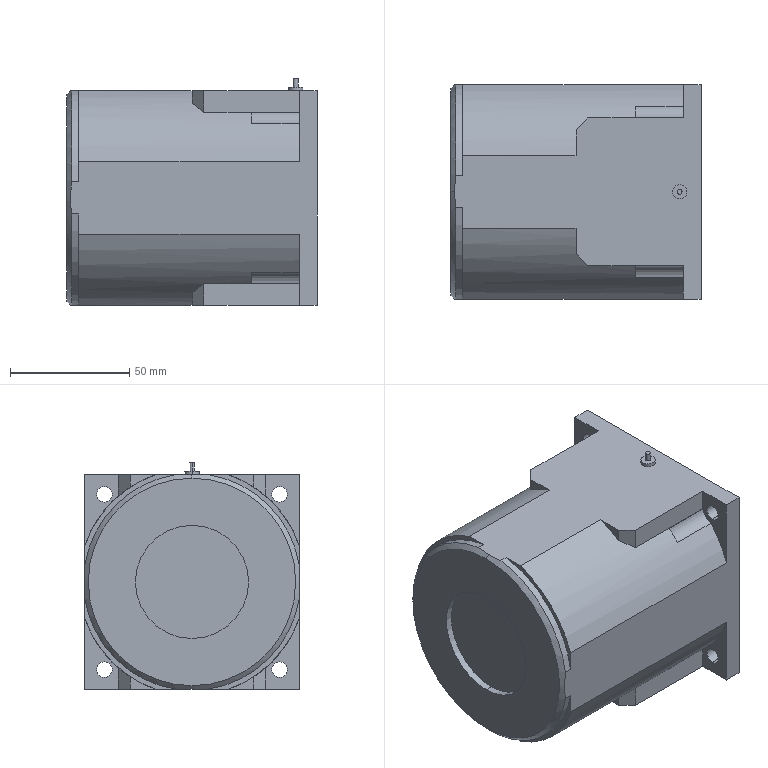Part | STEP file | 0230_Z_013_PACMR90-W40-V100-MTB90_1 | 1 solid | 61 faces | box 105 x 90 x 95 mm | volume 733234 mm3 | plane 33 | cylinder 26 | cone 2 | commonest cylinder face diameters 6.5 x8 11.5 x4 91 x4 95 x4 2 x2 6 x2